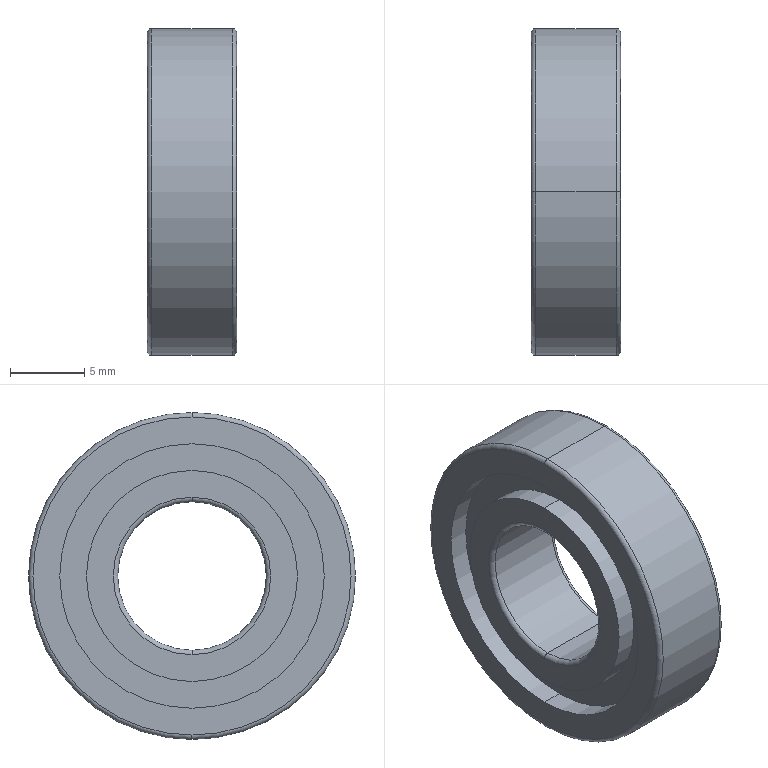Part | STEP file | B6900ZZ_B6900 | 1 solid | 26 faces | box 6 x 22 x 22 mm | volume 1551 mm3 | cylinder 12 | torus 8 | plane 6 | commonest cylinder face diameters 14.2 x4 17.8 x4 10 x2 22 x2